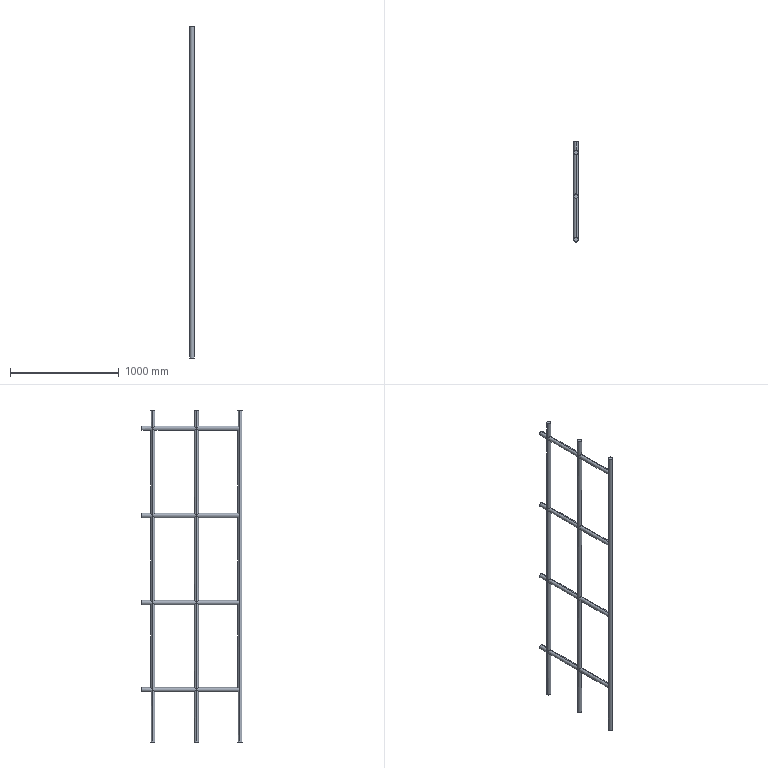Part | NX | features BREP 1 | 1 solid | 84 faces | box 40 x 920 x 3049 mm | volume 15567886 mm3 | cylinder 50 | plane 34 | commonest cylinder face diameters 40 x50